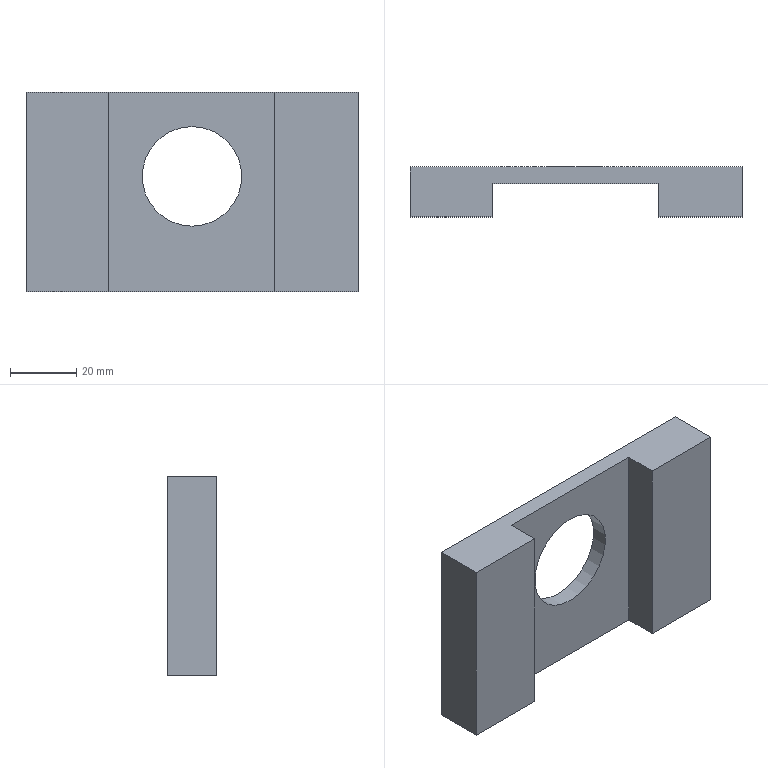Part | NX | features pneumatic support 2 | 1 solid | 11 faces | box 100 x 15 x 60 mm | volume 56466 mm3 | plane 10 | cylinder 1 | commonest cylinder face diameters 30 x1
STEP:
#1=CARTESIAN_POINT('',(200.,-100.,60.));
#2=VERTEX_POINT('',#1);
#3=CARTESIAN_POINT('',(200.,-110.,60.));
#4=VERTEX_POINT('',#3);
#5=CARTESIAN_POINT('',(200.,-110.,60.));
#6=DIRECTION('',(0.,1.,0.));
#7=VECTOR('',#6,1000.);
#8=LINE('',#5,#7);
#9=EDGE_CURVE('',#2,#4,#8,.F.);
#10=ORIENTED_EDGE('',*,*,#9,.F.);
#11=CARTESIAN_POINT('',(200.,-100.,0.));
#12=VERTEX_POINT('',#11);
#13=CARTESIAN_POINT('',(200.,-100.,-120.));
#14=DIRECTION('',(0.,0.,1.));
#15=VECTOR('',#14,1000.);
#16=LINE('',#13,#15);
#17=EDGE_CURVE('',#2,#12,#16,.F.);
#18=ORIENTED_EDGE('',*,*,#17,.T.);
#19=CARTESIAN_POINT('',(200.,-110.,0.));
#20=VERTEX_POINT('',#19);
#21=CARTESIAN_POINT('',(200.,-110.,0.));
#22=DIRECTION('',(0.,1.,0.));
#23=VECTOR('',#22,1000.);
#24=LINE('',#21,#23);
#25=EDGE_CURVE('',#12,#20,#24,.F.);
#26=ORIENTED_EDGE('',*,*,#25,.T.);
#27=CARTESIAN_POINT('',(200.,-110.,60.));
#28=DIRECTION('',(0.,0.,1.));
#29=VECTOR('',#28,1000.);
#30=LINE('',#27,#29);
#31=EDGE_CURVE('',#20,#4,#30,.T.);
#32=ORIENTED_EDGE('',*,*,#31,.T.);
#33=EDGE_LOOP('',(#10,#18,#26,#32));
#34=FACE_BOUND('',#33,.T.);
#35=CARTESIAN_POINT('',(200.,-110.,-120.));
#36=DIRECTION('',(1.,0.,0.));
#37=DIRECTION('',(0.,0.,-1.));
#38=AXIS2_PLACEMENT_3D('',#35,#36,#37);
#39=PLANE('',#38);
#40=ADVANCED_FACE('',(#34),#39,.F.);
#41=ORIENTED_EDGE('',*,*,#31,.F.);
#42=CARTESIAN_POINT('',(225.,-110.,0.));
#43=VERTEX_POINT('',#42);
#44=CARTESIAN_POINT('',(125.,-110.,0.));
#45=DIRECTION('',(1.,0.,0.));
#46=VECTOR('',#45,1000.);
#47=LINE('',#44,#46);
#48=EDGE_CURVE('',#20,#43,#47,.T.);
#49=ORIENTED_EDGE('',*,*,#48,.T.);
#50=CARTESIAN_POINT('',(225.,-110.,60.));
#51=VERTEX_POINT('',#50);
#52=CARTESIAN_POINT('',(225.,-110.,60.));
#53=DIRECTION('',(0.,0.,1.));
#54=VECTOR('',#53,1000.);
#55=LINE('',#52,#54);
#56=EDGE_CURVE('',#43,#51,#55,.T.);
#57=ORIENTED_EDGE('',*,*,#56,.T.);
#58=CARTESIAN_POINT('',(125.,-110.,60.));
#59=DIRECTION('',(1.,0.,0.));
#60=VECTOR('',#59,1000.);
#61=LINE('',#58,#60);
#62=EDGE_CURVE('',#4,#51,#61,.T.);
#63=ORIENTED_EDGE('',*,*,#62,.F.);
#64=EDGE_LOOP('',(#41,#49,#57,#63));
#65=FACE_BOUND('',#64,.T.);
#66=CARTESIAN_POINT('',(125.,-110.,60.));
#67=DIRECTION('',(0.,1.,0.));
#68=DIRECTION('',(0.,0.,1.));
#69=AXIS2_PLACEMENT_3D('',#66,#67,#68);
#70=PLANE('',#69);
#71=ADVANCED_FACE('',(#65),#70,.F.);
#72=CARTESIAN_POINT('',(150.,-110.,0.));
#73=VERTEX_POINT('',#72);
#74=CARTESIAN_POINT('',(150.,-110.,60.));
#75=VERTEX_POINT('',#74);
#76=CARTESIAN_POINT('',(150.,-110.,-120.));
#77=DIRECTION('',(0.,0.,1.));
#78=VECTOR('',#77,1000.);
#79=LINE('',#76,#78);
#80=EDGE_CURVE('',#73,#75,#79,.T.);
#81=ORIENTED_EDGE('',*,*,#80,.T.);
#82=CARTESIAN_POINT('',(125.,-110.,60.));
#83=VERTEX_POINT('',#82);
#84=CARTESIAN_POINT('',(125.,-110.,60.));
#85=DIRECTION('',(1.,0.,0.));
#86=VECTOR('',#85,1000.);
#87=LINE('',#84,#86);
#88=EDGE_CURVE('',#83,#75,#87,.T.);
#89=ORIENTED_EDGE('',*,*,#88,.F.);
#90=CARTESIAN_POINT('',(125.,-110.,0.));
#91=VERTEX_POINT('',#90);
#92=CARTESIAN_POINT('',(125.,-110.,60.));
#93=DIRECTION('',(0.,0.,-1.));
#94=VECTOR('',#93,1000.);
#95=LINE('',#92,#94);
#96=EDGE_CURVE('',#83,#91,#95,.T.);
#97=ORIENTED_EDGE('',*,*,#96,.T.);
#98=CARTESIAN_POINT('',(125.,-110.,0.));
#99=DIRECTION('',(1.,0.,0.));
#100=VECTOR('',#99,1000.);
#101=LINE('',#98,#100);
#102=EDGE_CURVE('',#91,#73,#101,.T.);
#103=ORIENTED_EDGE('',*,*,#102,.T.);
#104=EDGE_LOOP('',(#81,#89,#97,#103));
#105=FACE_BOUND('',#104,.T.);
#106=CARTESIAN_POINT('',(125.,-110.,60.));
#107=DIRECTION('',(0.,1.,0.));
#108=DIRECTION('',(0.,0.,1.));
#109=AXIS2_PLACEMENT_3D('',#106,#107,#108);
#110=PLANE('',#109);
#111=ADVANCED_FACE('',(#105),#110,.F.);
#112=CARTESIAN_POINT('',(150.,-100.,60.));
#113=VERTEX_POINT('',#112);
#114=CARTESIAN_POINT('',(150.,-110.,60.));
#115=DIRECTION('',(0.,1.,0.));
#116=VECTOR('',#115,1000.);
#117=LINE('',#114,#116);
#118=EDGE_CURVE('',#75,#113,#117,.T.);
#119=ORIENTED_EDGE('',*,*,#118,.F.);
#120=ORIENTED_EDGE('',*,*,#80,.F.);
#121=CARTESIAN_POINT('',(150.,-100.,0.));
#122=VERTEX_POINT('',#121);
#123=CARTESIAN_POINT('',(150.,-110.,0.));
#124=DIRECTION('',(0.,1.,0.));
#125=VECTOR('',#124,1000.);
#126=LINE('',#123,#125);
#127=EDGE_CURVE('',#73,#122,#126,.T.);
#128=ORIENTED_EDGE('',*,*,#127,.T.);
#129=CARTESIAN_POINT('',(150.,-100.,-120.));
#130=DIRECTION('',(0.,0.,1.));
#131=VECTOR('',#130,1000.);
#132=LINE('',#129,#131);
#133=EDGE_CURVE('',#122,#113,#132,.T.);
#134=ORIENTED_EDGE('',*,*,#133,.T.);
#135=EDGE_LOOP('',(#119,#120,#128,#134));
#136=FACE_BOUND('',#135,.T.);
#137=CARTESIAN_POINT('',(150.,-110.,-120.));
#138=DIRECTION('',(-1.,0.,0.));
#139=DIRECTION('',(0.,0.,1.));
#140=AXIS2_PLACEMENT_3D('',#137,#138,#139);
#141=PLANE('',#140);
#142=ADVANCED_FACE('',(#136),#141,.F.);
#143=CARTESIAN_POINT('',(125.,-100.,60.));
#144=DIRECTION('',(1.,0.,0.));
#145=VECTOR('',#144,1000.);
#146=LINE('',#143,#145);
#147=EDGE_CURVE('',#113,#2,#146,.T.);
#148=ORIENTED_EDGE('',*,*,#147,.F.);
#149=ORIENTED_EDGE('',*,*,#133,.F.);
#150=CARTESIAN_POINT('',(125.,-100.,0.));
#151=DIRECTION('',(1.,0.,0.));
#152=VECTOR('',#151,1000.);
#153=LINE('',#150,#152);
#154=EDGE_CURVE('',#122,#12,#153,.T.);
#155=ORIENTED_EDGE('',*,*,#154,.T.);
#156=ORIENTED_EDGE('',*,*,#17,.F.);
#157=EDGE_LOOP('',(#148,#149,#155,#156));
#158=FACE_BOUND('',#157,.T.);
#159=CARTESIAN_POINT('',(175.,-100.,49.7));
#160=VERTEX_POINT('',#159);
#161=CARTESIAN_POINT('',(175.,-100.,34.7));
#162=DIRECTION('',(0.,1.,0.));
#163=DIRECTION('',(0.,0.,1.));
#164=AXIS2_PLACEMENT_3D('',#161,#162,#163);
#165=CIRCLE('',#164,15.);
#166=EDGE_CURVE('',#160,#160,#165,.T.);
#167=ORIENTED_EDGE('',*,*,#166,.T.);
#168=EDGE_LOOP('',(#167));
#169=FACE_BOUND('',#168,.T.);
#170=CARTESIAN_POINT('',(150.,-100.,-120.));
#171=DIRECTION('',(0.,1.,0.));
#172=DIRECTION('',(0.,0.,1.));
#173=AXIS2_PLACEMENT_3D('',#170,#171,#172);
#174=PLANE('',#173);
#175=ADVANCED_FACE('',(#158,#169),#174,.F.);
#176=ORIENTED_EDGE('',*,*,#166,.F.);
#177=EDGE_LOOP('',(#176));
#178=FACE_BOUND('',#177,.T.);
#179=CARTESIAN_POINT('',(175.,-95.,49.7));
#180=VERTEX_POINT('',#179);
#181=CARTESIAN_POINT('',(175.,-95.,34.7));
#182=DIRECTION('',(0.,1.,0.));
#183=DIRECTION('',(0.,0.,1.));
#184=AXIS2_PLACEMENT_3D('',#181,#182,#183);
#185=CIRCLE('',#184,15.);
#186=EDGE_CURVE('',#180,#180,#185,.T.);
#187=ORIENTED_EDGE('',*,*,#186,.T.);
#188=EDGE_LOOP('',(#187));
#189=FACE_BOUND('',#188,.T.);
#190=CARTESIAN_POINT('',(175.,-155.,34.7));
#191=DIRECTION('',(0.,1.,0.));
#192=DIRECTION('',(0.,0.,1.));
#193=AXIS2_PLACEMENT_3D('',#190,#191,#192);
#194=CYLINDRICAL_SURFACE('',#193,15.);
#195=ADVANCED_FACE('',(#178,#189),#194,.F.);
#196=CARTESIAN_POINT('',(225.,-95.,0.));
#197=VERTEX_POINT('',#196);
#198=CARTESIAN_POINT('',(225.,-95.,60.));
#199=VERTEX_POINT('',#198);
#200=CARTESIAN_POINT('',(225.,-95.,60.));
#201=DIRECTION('',(0.,0.,-1.));
#202=VECTOR('',#201,1000.);
#203=LINE('',#200,#202);
#204=EDGE_CURVE('',#197,#199,#203,.F.);
#205=ORIENTED_EDGE('',*,*,#204,.T.);
#206=CARTESIAN_POINT('',(225.,-110.,60.));
#207=DIRECTION('',(0.,1.,0.));
#208=VECTOR('',#207,1000.);
#209=LINE('',#206,#208);
#210=EDGE_CURVE('',#51,#199,#209,.T.);
#211=ORIENTED_EDGE('',*,*,#210,.F.);
#212=ORIENTED_EDGE('',*,*,#56,.F.);
#213=CARTESIAN_POINT('',(225.,-110.,0.));
#214=DIRECTION('',(0.,1.,0.));
#215=VECTOR('',#214,1000.);
#216=LINE('',#213,#215);
#217=EDGE_CURVE('',#43,#197,#216,.T.);
#218=ORIENTED_EDGE('',*,*,#217,.T.);
#219=EDGE_LOOP('',(#205,#211,#212,#218));
#220=FACE_BOUND('',#219,.T.);
#221=CARTESIAN_POINT('',(225.,-95.,60.));
#222=DIRECTION('',(-1.,0.,0.));
#223=DIRECTION('',(0.,-1.,0.));
#224=AXIS2_PLACEMENT_3D('',#221,#222,#223);
#225=PLANE('',#224);
#226=ADVANCED_FACE('',(#220),#225,.F.);
#227=CARTESIAN_POINT('',(125.,-95.,60.));
#228=VERTEX_POINT('',#227);
#229=CARTESIAN_POINT('',(125.,-95.,60.));
#230=DIRECTION('',(0.,1.,0.));
#231=VECTOR('',#230,1000.);
#232=LINE('',#229,#231);
#233=EDGE_CURVE('',#228,#83,#232,.F.);
#234=ORIENTED_EDGE('',*,*,#233,.T.);
#235=ORIENTED_EDGE('',*,*,#88,.T.);
#236=ORIENTED_EDGE('',*,*,#118,.T.);
#237=ORIENTED_EDGE('',*,*,#147,.T.);
#238=ORIENTED_EDGE('',*,*,#9,.T.);
#239=ORIENTED_EDGE('',*,*,#62,.T.);
#240=ORIENTED_EDGE('',*,*,#210,.T.);
#241=CARTESIAN_POINT('',(125.,-95.,60.));
#242=DIRECTION('',(1.,0.,0.));
#243=VECTOR('',#242,1000.);
#244=LINE('',#241,#243);
#245=EDGE_CURVE('',#199,#228,#244,.F.);
#246=ORIENTED_EDGE('',*,*,#245,.T.);
#247=EDGE_LOOP('',(#234,#235,#236,#237,#238,#239,#240,#246));
#248=FACE_BOUND('',#247,.T.);
#249=CARTESIAN_POINT('',(125.,-110.,60.));
#250=DIRECTION('',(0.,0.,1.));
#251=DIRECTION('',(1.,0.,0.));
#252=AXIS2_PLACEMENT_3D('',#249,#250,#251);
#253=PLANE('',#252);
#254=ADVANCED_FACE('',(#248),#253,.T.);
#255=ORIENTED_EDGE('',*,*,#96,.F.);
#256=ORIENTED_EDGE('',*,*,#233,.F.);
#257=CARTESIAN_POINT('',(125.,-95.,0.));
#258=VERTEX_POINT('',#257);
#259=CARTESIAN_POINT('',(125.,-95.,60.));
#260=DIRECTION('',(0.,0.,-1.));
#261=VECTOR('',#260,1000.);
#262=LINE('',#259,#261);
#263=EDGE_CURVE('',#228,#258,#262,.T.);
#264=ORIENTED_EDGE('',*,*,#263,.T.);
#265=CARTESIAN_POINT('',(125.,-110.,0.));
#266=DIRECTION('',(0.,1.,0.));
#267=VECTOR('',#266,1000.);
#268=LINE('',#265,#267);
#269=EDGE_CURVE('',#258,#91,#268,.F.);
#270=ORIENTED_EDGE('',*,*,#269,.T.);
#271=EDGE_LOOP('',(#255,#256,#264,#270));
#272=FACE_BOUND('',#271,.T.);
#273=CARTESIAN_POINT('',(125.,-95.,60.));
#274=DIRECTION('',(1.,0.,0.));
#275=DIRECTION('',(0.,0.,-1.));
#276=AXIS2_PLACEMENT_3D('',#273,#274,#275);
#277=PLANE('',#276);
#278=ADVANCED_FACE('',(#272),#277,.F.);
#279=ORIENTED_EDGE('',*,*,#127,.F.);
#280=ORIENTED_EDGE('',*,*,#102,.F.);
#281=ORIENTED_EDGE('',*,*,#269,.F.);
#282=CARTESIAN_POINT('',(125.,-95.,0.));
#283=DIRECTION('',(1.,0.,0.));
#284=VECTOR('',#283,1000.);
#285=LINE('',#282,#284);
#286=EDGE_CURVE('',#258,#197,#285,.T.);
#287=ORIENTED_EDGE('',*,*,#286,.T.);
#288=ORIENTED_EDGE('',*,*,#217,.F.);
#289=ORIENTED_EDGE('',*,*,#48,.F.);
#290=ORIENTED_EDGE('',*,*,#25,.F.);
#291=ORIENTED_EDGE('',*,*,#154,.F.);
#292=EDGE_LOOP('',(#279,#280,#281,#287,#288,#289,#290,#291));
#293=FACE_BOUND('',#292,.T.);
#294=CARTESIAN_POINT('',(125.,-110.,0.));
#295=DIRECTION('',(0.,0.,1.));
#296=DIRECTION('',(1.,0.,0.));
#297=AXIS2_PLACEMENT_3D('',#294,#295,#296);
#298=PLANE('',#297);
#299=ADVANCED_FACE('',(#293),#298,.F.);
#300=ORIENTED_EDGE('',*,*,#263,.F.);
#301=ORIENTED_EDGE('',*,*,#245,.F.);
#302=ORIENTED_EDGE('',*,*,#204,.F.);
#303=ORIENTED_EDGE('',*,*,#286,.F.);
#304=EDGE_LOOP('',(#300,#301,#302,#303));
#305=FACE_BOUND('',#304,.T.);
#306=ORIENTED_EDGE('',*,*,#186,.F.);
#307=EDGE_LOOP('',(#306));
#308=FACE_BOUND('',#307,.T.);
#309=CARTESIAN_POINT('',(125.,-95.,60.));
#310=DIRECTION('',(0.,-1.,0.));
#311=DIRECTION('',(0.,0.,-1.));
#312=AXIS2_PLACEMENT_3D('',#309,#310,#311);
#313=PLANE('',#312);
#314=ADVANCED_FACE('',(#305,#308),#313,.F.);
#315=CLOSED_SHELL('',(#40,#71,#111,#142,#175,#195,#226,#254,#278,#299,#314));
#316=MANIFOLD_SOLID_BREP('',#315);
#317=(LENGTH_UNIT()NAMED_UNIT(*)SI_UNIT(.MILLI.,.METRE.));
#318=UNCERTAINTY_MEASURE_WITH_UNIT(LENGTH_MEASURE(0.00001),#317,'','');
#319=(NAMED_UNIT(*)PLANE_ANGLE_UNIT()SI_UNIT($,.RADIAN.));
#320=(NAMED_UNIT(*)SI_UNIT($,.STERADIAN.)SOLID_ANGLE_UNIT());
#321=(GEOMETRIC_REPRESENTATION_CONTEXT(3)GLOBAL_UNCERTAINTY_ASSIGNED_CONTEXT((#318))GLOBAL_UNIT_ASSIGNED_CONTEXT((#317,#319,#320))REPRESENTATION_CONTEXT('',''));
#322=ADVANCED_BREP_SHAPE_REPRESENTATION('',(#316),#321);